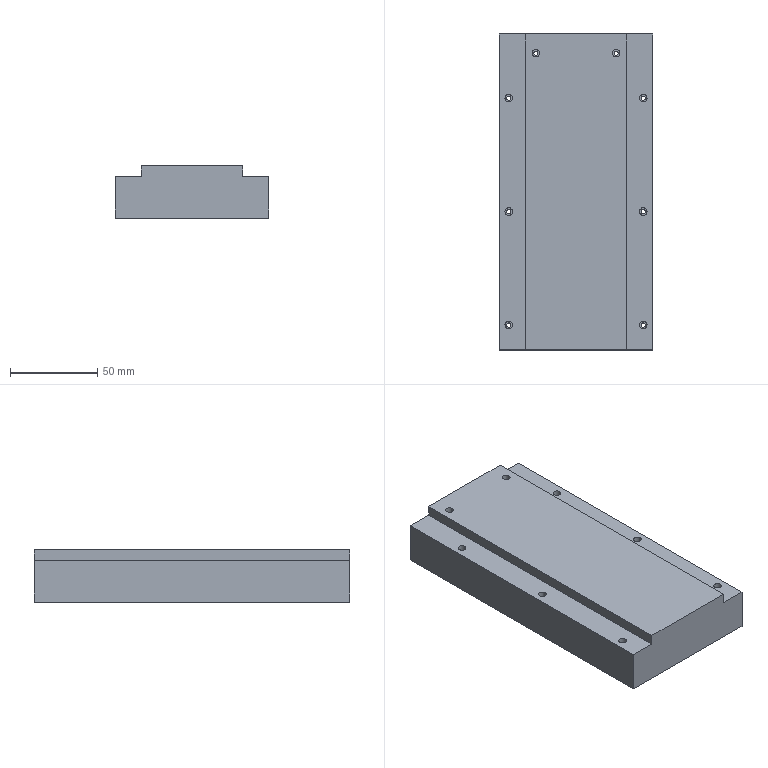NC program | NX | posted with a generic post | part box 88 x 181.05 x 30 mm
Lines 5406 to 5444 of 7800:
(PLANAR_MILL_9_COPY , TOOL : D12-36-D12-120-3T-FINISH)
N10810 T03 M6
N10812 G54
N10814 G17 G0 G90 X53.649 Y-84.525 B0. C0. S3500 M3
N10816 G43 Z44.5 H3
N10818 Z5.55
N10820 G94 G1 Z2.55 F800.
N10822 X41.649
N10824 X-41.649
N10826 X-53.649
N10828 Z5.55
N10830 G0 Z44.5
(PLANAR_MILL_9_COPY_COPY_1 , TOOL : D12-36-D12-120-3T-FINISH)
N10832 Z54.55
N10834 X-5. Y53.649
N10836 Z5.55
N10838 G1 Z2.55
N10840 Y41.649
N10842 Y-41.649
N10844 Y-53.649
N10846 Z5.55
N10848 G0 Z54.55
(PLANAR_MILL_9 , TOOL : D12-36-D12-120-3T-FINISH)
N10850 X53.649 Y-84.525
N10852 Z44.5
N10854 Z5.5
N10856 G1 Z2.5
N10858 X41.649
N10860 X-41.649
N10862 X-53.649
N10864 Z5.5
N10866 G0 Z44.5
N10868 M5